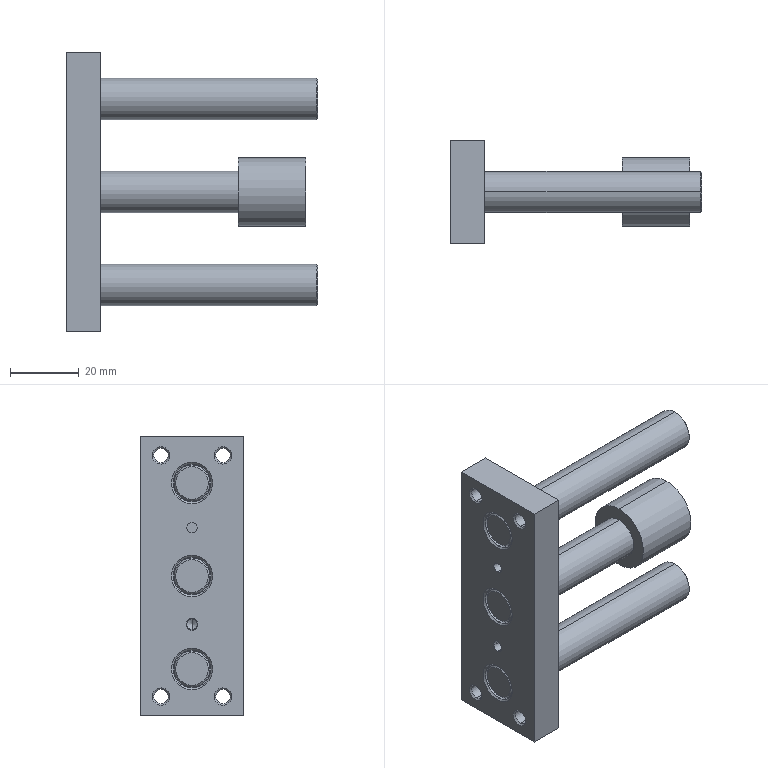Part | STEP file | 11-_TCM-20x20-0_20fp11 | 1 solid | 90 faces | box 73 x 30 x 81 mm | volume 48247 mm3 | cylinder 35 | cone 34 | plane 21 | commonest cylinder face diameters 4.134 x8 3 x7 10.5 x6 11 x6 12 x6 19.9 x2